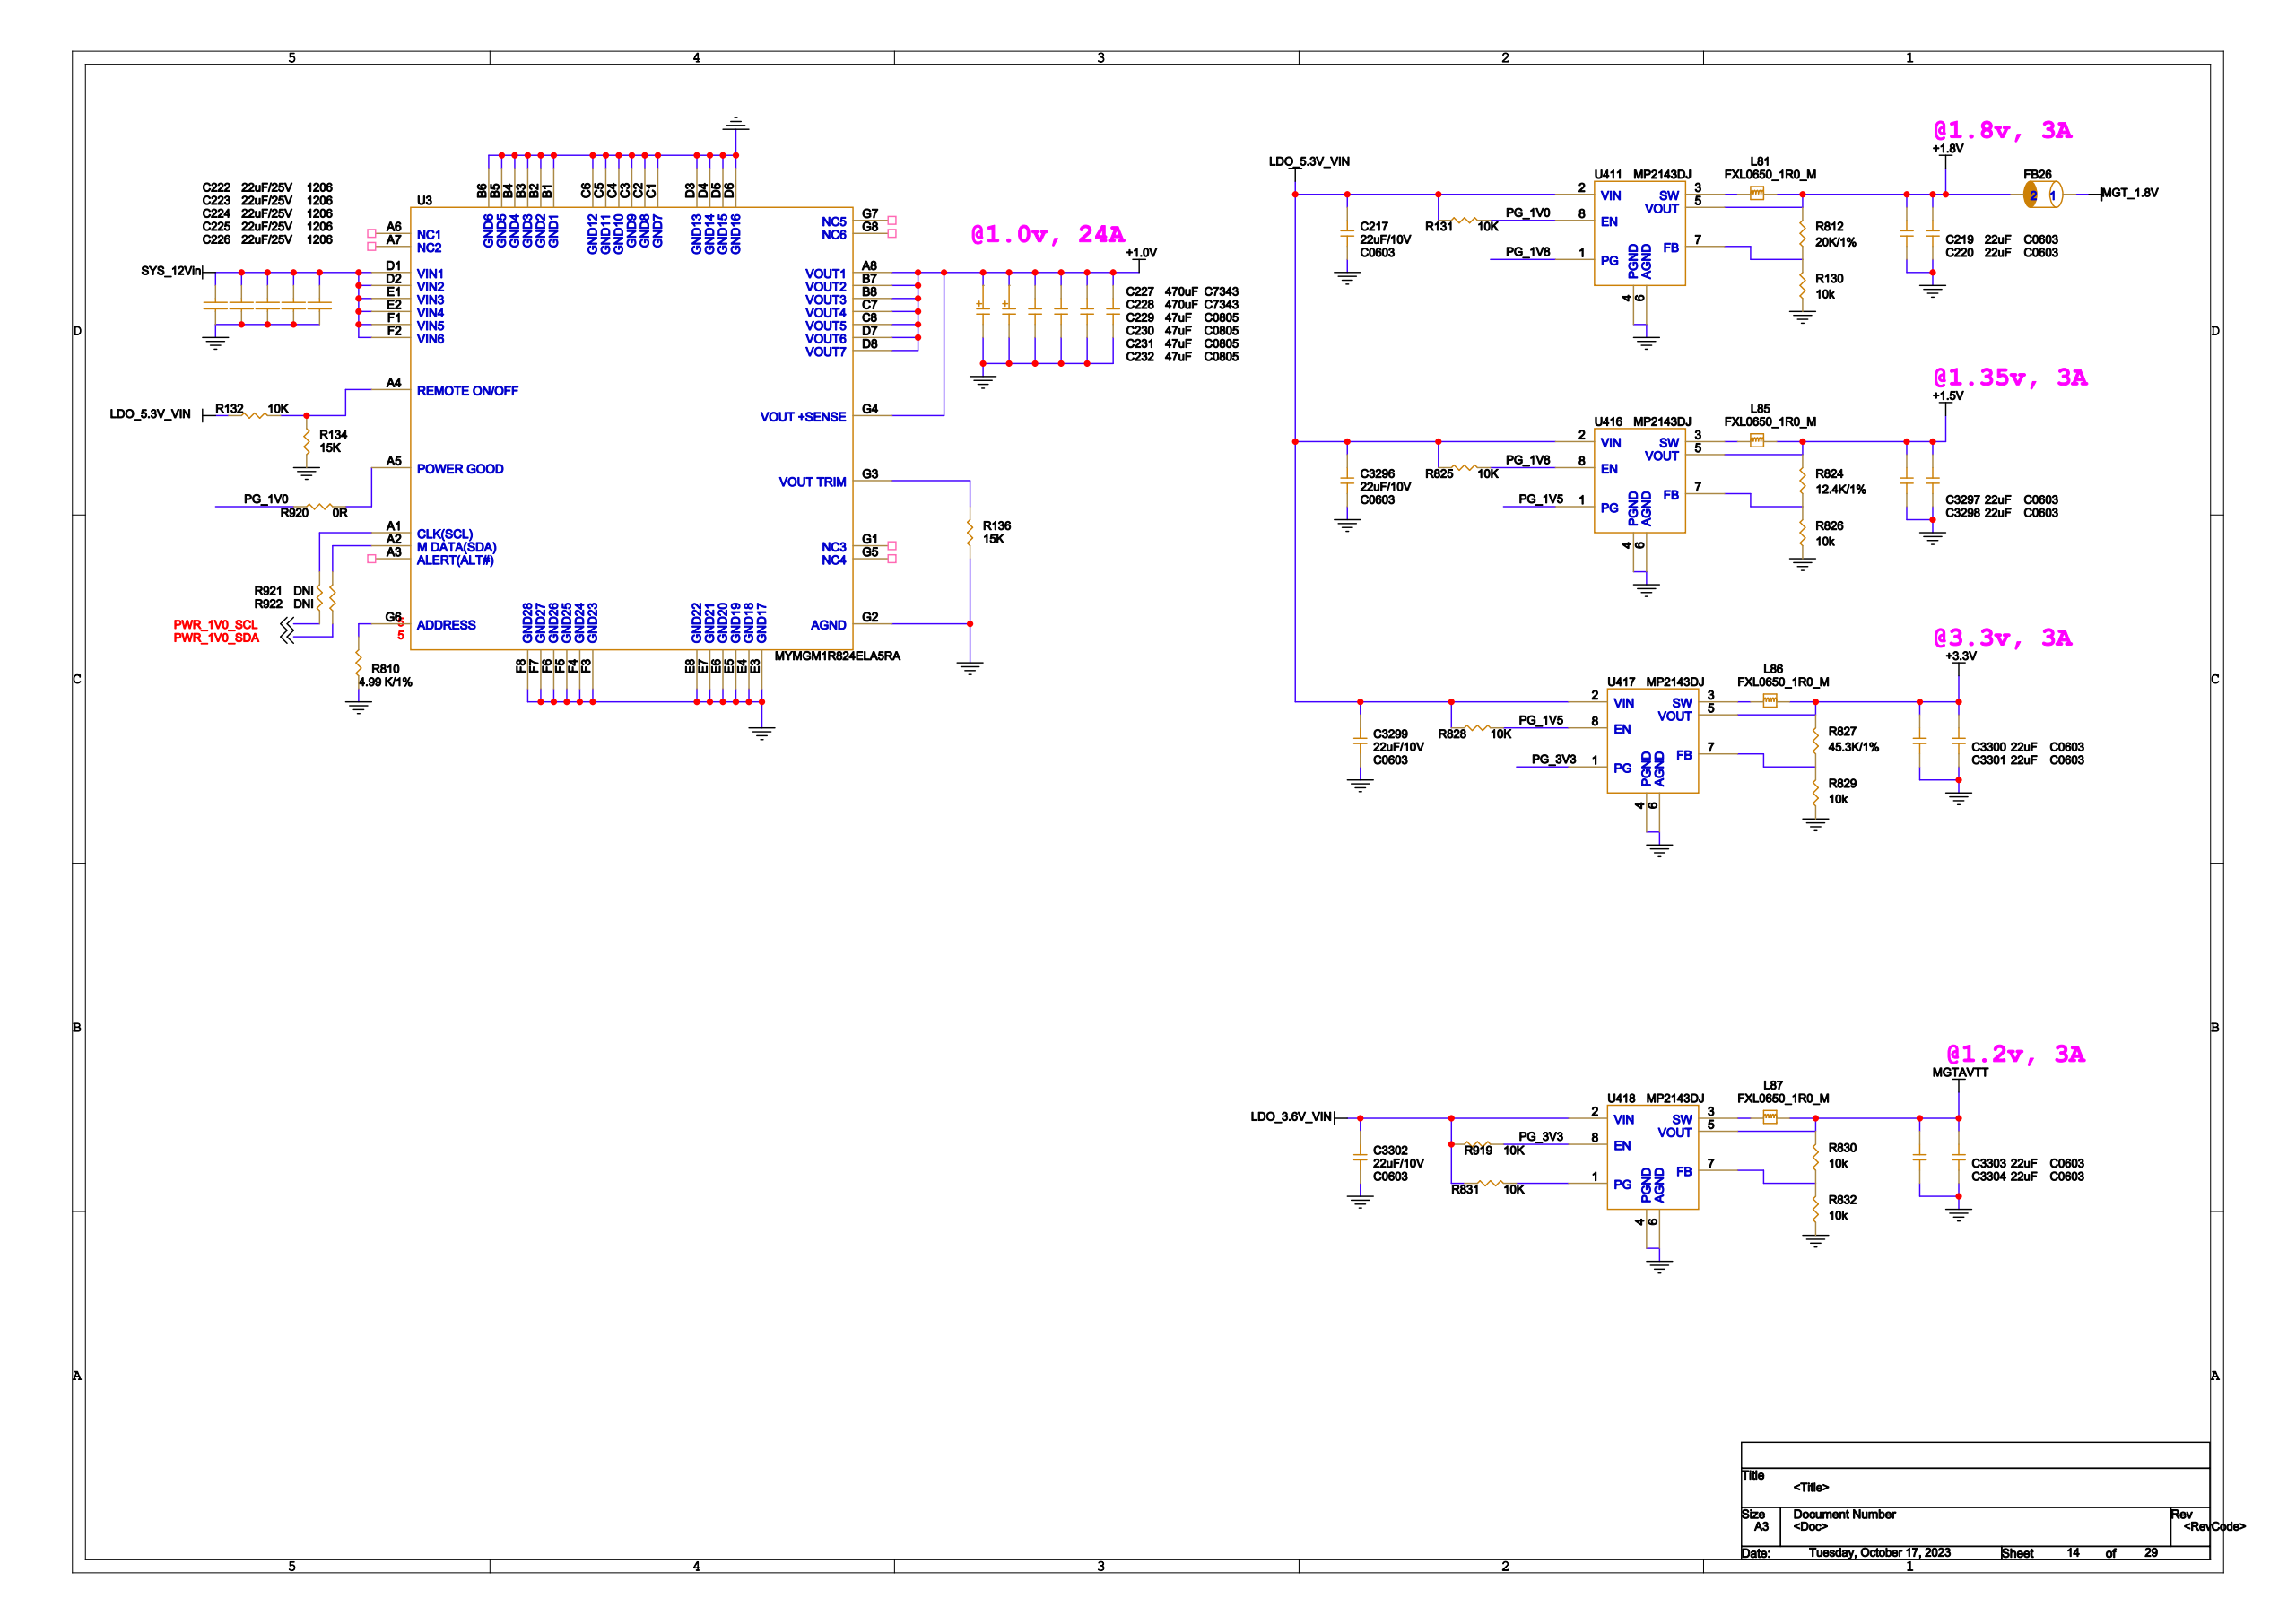Circuit board | Cadence Allegro | 1793 parts | 1223 nets | one sheet of the schematic
Parts on this sheet (reference | value | footprint):
C217 | 22uF/10V | C0603
C219 | 22uF | C0603
C220 | 22uF | C0603
C222 | 22uF/25V | 1206
C223 | 22uF/25V | 1206
C224 | 22uF/25V | 1206
C225 | 22uF/25V | 1206
C226 | 22uF/25V | 1206
C227 | 470uF | C7343
C228 | 470uF | C7343
C229 | 47uF | C0805
C230 | 47uF | C0805
C231 | 47uF | C0805
C232 | 47uF | C0805
C3296 | 22uF/10V | C0603
C3297 | 22uF | C0603
C3298 | 22uF | C0603
C3299 | 22uF/10V | C0603
C3300 | 22uF | C0603
C3301 | 22uF | C0603
C3302 | 22uF/10V | C0603
C3303 | 22uF | C0603
C3304 | 22uF | C0603
FB26 | BLM18PG121SN1 | FB0603
L81 | FXL0650_1R0_M | SMD_SMD_7X6_6
L85 | FXL0650_1R0_M | SMD_SMD_7X6_6
L86 | FXL0650_1R0_M | SMD_SMD_7X6_6
L87 | FXL0650_1R0_M | SMD_SMD_7X6_6
R130 | 10k | R0402
R131 | 10k | R0402
R132 | 10k | R0402
R134 | 15K | R0402
R136 | 15K | R0402
R810 | 4.99 K/1% | R0402
R812 | 20K/1% | R0402
R824 | 12.4K/1% | R0402
R825 | 10k | R0402
R826 | 10k | R0402
R827 | 45.3K/1% | R0402
R828 | 10k | R0402
R829 | 10k | R0402
R830 | 10k | R0402
R831 | 10k | R0402
R832 | 10k | R0402
R919 | 10k | R0402
R920 | 0R | R0402
R921 | DNI | R0402
R922 | DNI | R0402
U3 | MYMGM1R824ELA5RA | MYMGM1R
U411 | MP2143DJ | SOT-23-8
U416 | MP2143DJ | SOT-23-8
U417 | MP2143DJ | SOT-23-8
U418 | MP2143DJ | SOT-23-8
Nets of these parts (net: part-pin ...):
GND: C217-1 C219-1 C220-1 C222-1 C223-1 C224-1 C225-1 C226-1 C227-2 C228-2 C229-1 C230-1 C231-1 C232-1 C3296-1 C3297-1 C3298-1 C3299-1 C3300-1 C3301-1 C3302-1 C3303-1 C3304-1 R130-2 R134-1 R136-2 R810-2 R826-2 R829-2 R832-2 U411-4 U411-6 U416-4 U416-6 U417-4 U417-6 U418-4 U418-6 U3-B1 U3-B2 U3-B3 U3-B4 U3-B5 U3-B6 U3-C1 U3-C2 U3-C3 U3-C4 U3-C5 U3-C6 U3-D3 U3-D4 U3-D5 U3-D6 U3-E3 U3-E4 U3-E5 U3-E6 U3-E7 U3-E8 U3-F3 U3-F4 U3-F5 U3-F6 U3-F7 U3-F8 U3-G2
+1.5V: C3297-2 C3298-2 L85-2 R824-1 U416-5
+3.3V: C3300-2 C3301-2 L86-2 R827-1 U417-5
N16833646: R130-1 R812-2 U411-7
PG_1V0: R131-1 R920-2 U411-8
LDO_5.3V_VIN: C217-2 C3296-2 C3299-2 R131-2 R132-2 R825-2 R828-2 U411-2 U416-2 U417-2
N16819890: R132-1 R134-2 U3-A4
SYS_12VIN: C222-2 C223-2 C224-2 C225-2 C226-2 U3-D1 U3-D2 U3-E1 U3-E2 U3-F1 U3-F2
PG_1V8: R825-1 U411-1 U416-8
N16837392: R824-2 R826-1 U416-7
PG_1V5: R828-1 U416-1 U417-8
N16838590: R827-2 R829-1 U417-7
MGTAVTT: C3303-2 C3304-2 L87-2 R830-1 U418-5
N16839962: R830-2 R832-1 U418-7
N16839970: R831-1 U418-1
LDO_3.6V_VIN: C3302-2 R831-2 R919-2 U418-2
PG_3V3: R919-1 U417-1 U418-8
+1.0V: C227-1 C228-1 C229-2 C230-2 C231-2 C232-2 U3-A8 U3-B7 U3-B8 U3-C7 U3-C8 U3-D7 U3-D8 U3-G4
+1.8V: C219-2 C220-2 FB26-2 L81-2 R812-1 U411-5
MGT_1.8V: FB26-1
N16819946: R810-1 U3-G6
N16824356: L81-1 U411-3
N16837313: L85-1 U416-3
N16838511: L86-1 U417-3
N16839883: L87-1 U418-3
N16819926: R136-1 U3-G3
N16963100: R920-1 U3-A5
N17114755: R921-1 U3-A1
PWR_1V0_SCL: R921-2
N17114764: R922-1 U3-A2
PWR_1V0_SDA: R922-2